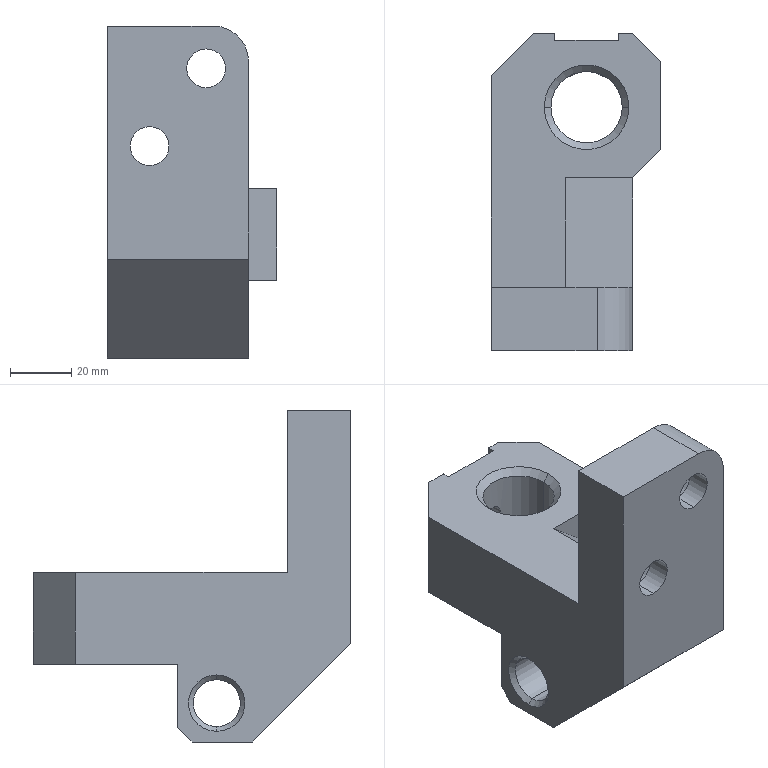Part | SolidWorks | features BaseBody 1 | 1 solid | 49 faces | box 55.385 x 103.846 x 108.462 mm | volume 199714 mm3 | plane 24 | cylinder 15 | cone 10 | commonest cylinder face diameters 23.077 x5 12.692 x4 5.675 x2 15.339 x2 23.322 x2